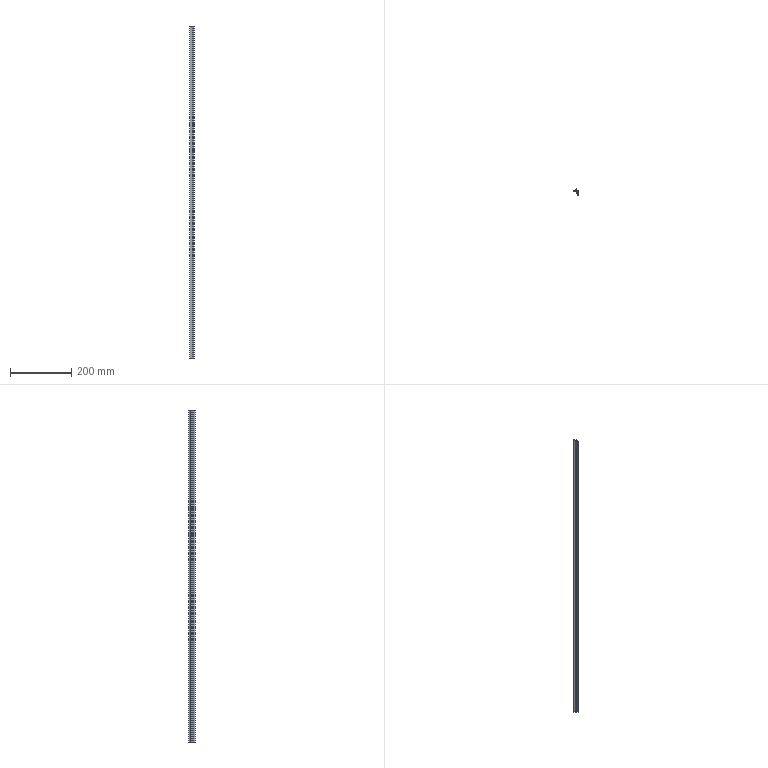Part | SolidWorks | features BaseBody 1, ICE 1, MoveFace 1 | 1 solid | 27 faces | box 14 x 20.3 x 1088 mm | volume 55396 mm3 | plane 20 | cylinder 7 | commonest cylinder face diameters 0.387 x2 0.8 x2 0.4 x1 20 x1 22 x1
STEP:
#1=CARTESIAN_POINT('',(-5.304,-0.625,200.));
#2=VERTEX_POINT('',#1);
#3=CARTESIAN_POINT('',(-5.449,-0.8125,200.));
#4=VERTEX_POINT('',#3);
#5=CARTESIAN_POINT('',(-5.255,-0.8125,200.));
#6=DIRECTION('',(0.,0.,1.));
#7=DIRECTION('',(-1.,0.,0.));
#8=AXIS2_PLACEMENT_3D('',#5,#6,#7);
#9=CIRCLE('',#8,0.1937);
#10=EDGE_CURVE('',#2,#4,#9,.T.);
#11=ORIENTED_EDGE('',*,*,#10,.T.);
#12=CARTESIAN_POINT('',(-5.449,-0.8125,-888.));
#13=VERTEX_POINT('',#12);
#14=CARTESIAN_POINT('',(-5.449,-0.8125,230.));
#15=DIRECTION('',(0.,0.,-1.));
#16=VECTOR('',#15,1000.);
#17=LINE('',#14,#16);
#18=EDGE_CURVE('',#4,#13,#17,.T.);
#19=ORIENTED_EDGE('',*,*,#18,.T.);
#20=CARTESIAN_POINT('',(-5.304,-0.625,-888.));
#21=VERTEX_POINT('',#20);
#22=CARTESIAN_POINT('',(-5.255,-0.8125,-888.));
#23=DIRECTION('',(0.,0.,-1.));
#24=DIRECTION('',(1.,0.,0.));
#25=AXIS2_PLACEMENT_3D('',#22,#23,#24);
#26=CIRCLE('',#25,0.1937);
#27=EDGE_CURVE('',#13,#21,#26,.T.);
#28=ORIENTED_EDGE('',*,*,#27,.T.);
#29=CARTESIAN_POINT('',(-5.304,-0.625,230.));
#30=DIRECTION('',(0.,0.,-1.));
#31=VECTOR('',#30,1000.);
#32=LINE('',#29,#31);
#33=EDGE_CURVE('',#2,#21,#32,.T.);
#34=ORIENTED_EDGE('',*,*,#33,.F.);
#35=EDGE_LOOP('',(#11,#19,#28,#34));
#36=FACE_OUTER_BOUND('',#35,.T.);
#37=CARTESIAN_POINT('',(-5.255,-0.8125,230.));
#38=DIRECTION('',(0.,0.,-1.));
#39=DIRECTION('',(-1.,0.,0.));
#40=AXIS2_PLACEMENT_3D('',#37,#38,#39);
#41=CYLINDRICAL_SURFACE('',#40,0.1937);
#42=ADVANCED_FACE('',(#36),#41,.F.);
#43=CARTESIAN_POINT('',(5.,-1.,-888.));
#44=VERTEX_POINT('',#43);
#45=CARTESIAN_POINT('',(5.,-14.3,-888.));
#46=VERTEX_POINT('',#45);
#47=CARTESIAN_POINT('',(5.,29.623,-888.));
#48=DIRECTION('',(0.,-1.,0.));
#49=VECTOR('',#48,1000.);
#50=LINE('',#47,#49);
#51=EDGE_CURVE('',#44,#46,#50,.T.);
#52=ORIENTED_EDGE('',*,*,#51,.F.);
#53=CARTESIAN_POINT('',(5.,-1.,200.));
#54=VERTEX_POINT('',#53);
#55=CARTESIAN_POINT('',(5.,-1.,230.));
#56=DIRECTION('',(0.,0.,-1.));
#57=VECTOR('',#56,1000.);
#58=LINE('',#55,#57);
#59=EDGE_CURVE('',#54,#44,#58,.T.);
#60=ORIENTED_EDGE('',*,*,#59,.F.);
#61=CARTESIAN_POINT('',(5.,-14.3,200.));
#62=VERTEX_POINT('',#61);
#63=CARTESIAN_POINT('',(5.,-14.3,200.));
#64=DIRECTION('',(0.,1.,0.));
#65=VECTOR('',#64,1000.);
#66=LINE('',#63,#65);
#67=EDGE_CURVE('',#62,#54,#66,.T.);
#68=ORIENTED_EDGE('',*,*,#67,.F.);
#69=CARTESIAN_POINT('',(5.,-14.3,230.));
#70=DIRECTION('',(0.,0.,1.));
#71=VECTOR('',#70,1000.);
#72=LINE('',#69,#71);
#73=EDGE_CURVE('',#46,#62,#72,.T.);
#74=ORIENTED_EDGE('',*,*,#73,.F.);
#75=EDGE_LOOP('',(#52,#60,#68,#74));
#76=FACE_OUTER_BOUND('',#75,.T.);
#77=CARTESIAN_POINT('',(5.,-14.3,230.));
#78=DIRECTION('',(-1.,0.,0.));
#79=DIRECTION('',(0.,0.,1.));
#80=AXIS2_PLACEMENT_3D('',#77,#78,#79);
#81=PLANE('',#80);
#82=ADVANCED_FACE('',(#76),#81,.F.);
#83=CARTESIAN_POINT('',(-9.,-2.,-888.));
#84=VERTEX_POINT('',#83);
#85=CARTESIAN_POINT('',(-9.,-2.,200.));
#86=VERTEX_POINT('',#85);
#87=CARTESIAN_POINT('',(-9.,-2.,230.));
#88=DIRECTION('',(0.,0.,1.));
#89=VECTOR('',#88,1000.);
#90=LINE('',#87,#89);
#91=EDGE_CURVE('',#84,#86,#90,.T.);
#92=ORIENTED_EDGE('',*,*,#91,.F.);
#93=CARTESIAN_POINT('',(0.9,-2.,-888.));
#94=VERTEX_POINT('',#93);
#95=CARTESIAN_POINT('',(5.,-2.,-888.));
#96=DIRECTION('',(-1.,0.,0.));
#97=VECTOR('',#96,1000.);
#98=LINE('',#95,#97);
#99=EDGE_CURVE('',#94,#84,#98,.T.);
#100=ORIENTED_EDGE('',*,*,#99,.F.);
#101=CARTESIAN_POINT('',(0.9,-2.,200.));
#102=VERTEX_POINT('',#101);
#103=CARTESIAN_POINT('',(0.9,-2.,230.));
#104=DIRECTION('',(0.,0.,-1.));
#105=VECTOR('',#104,1000.);
#106=LINE('',#103,#105);
#107=EDGE_CURVE('',#102,#94,#106,.T.);
#108=ORIENTED_EDGE('',*,*,#107,.F.);
#109=CARTESIAN_POINT('',(5.,-2.,200.));
#110=DIRECTION('',(1.,0.,0.));
#111=VECTOR('',#110,1000.);
#112=LINE('',#109,#111);
#113=EDGE_CURVE('',#86,#102,#112,.T.);
#114=ORIENTED_EDGE('',*,*,#113,.F.);
#115=EDGE_LOOP('',(#92,#100,#108,#114));
#116=FACE_OUTER_BOUND('',#115,.T.);
#117=CARTESIAN_POINT('',(-9.,-2.,230.));
#118=DIRECTION('',(0.,1.,0.));
#119=DIRECTION('',(0.,0.,1.));
#120=AXIS2_PLACEMENT_3D('',#117,#118,#119);
#121=PLANE('',#120);
#122=ADVANCED_FACE('',(#116),#121,.F.);
#123=CARTESIAN_POINT('',(4.,-6.,200.));
#124=VERTEX_POINT('',#123);
#125=CARTESIAN_POINT('',(4.,-3.,200.));
#126=VERTEX_POINT('',#125);
#127=CARTESIAN_POINT('',(4.,29.623,200.));
#128=DIRECTION('',(0.,1.,0.));
#129=VECTOR('',#128,1000.);
#130=LINE('',#127,#129);
#131=EDGE_CURVE('',#124,#126,#130,.T.);
#132=ORIENTED_EDGE('',*,*,#131,.F.);
#133=CARTESIAN_POINT('',(1.,-6.,200.));
#134=VERTEX_POINT('',#133);
#135=CARTESIAN_POINT('',(5.,-6.,200.));
#136=DIRECTION('',(1.,0.,0.));
#137=VECTOR('',#136,1000.);
#138=LINE('',#135,#137);
#139=EDGE_CURVE('',#134,#124,#138,.T.);
#140=ORIENTED_EDGE('',*,*,#139,.F.);
#141=CARTESIAN_POINT('',(1.,-6.7,200.));
#142=VERTEX_POINT('',#141);
#143=CARTESIAN_POINT('',(1.,-6.,200.));
#144=DIRECTION('',(0.,-1.,0.));
#145=VECTOR('',#144,1000.);
#146=LINE('',#143,#145);
#147=EDGE_CURVE('',#134,#142,#146,.T.);
#148=ORIENTED_EDGE('',*,*,#147,.T.);
#149=CARTESIAN_POINT('',(-1.7,-6.7,200.));
#150=VERTEX_POINT('',#149);
#151=CARTESIAN_POINT('',(5.,-6.7,200.));
#152=DIRECTION('',(1.,0.,0.));
#153=VECTOR('',#152,1000.);
#154=LINE('',#151,#153);
#155=EDGE_CURVE('',#150,#142,#154,.T.);
#156=ORIENTED_EDGE('',*,*,#155,.F.);
#157=CARTESIAN_POINT('',(-1.7,-7.7,200.));
#158=VERTEX_POINT('',#157);
#159=CARTESIAN_POINT('',(-1.7,-6.7,200.));
#160=DIRECTION('',(0.,-1.,0.));
#161=VECTOR('',#160,1000.);
#162=LINE('',#159,#161);
#163=EDGE_CURVE('',#150,#158,#162,.T.);
#164=ORIENTED_EDGE('',*,*,#163,.T.);
#165=CARTESIAN_POINT('',(4.,-7.7,200.));
#166=VERTEX_POINT('',#165);
#167=CARTESIAN_POINT('',(5.,-7.7,200.));
#168=DIRECTION('',(-1.,0.,0.));
#169=VECTOR('',#168,1000.);
#170=LINE('',#167,#169);
#171=EDGE_CURVE('',#166,#158,#170,.T.);
#172=ORIENTED_EDGE('',*,*,#171,.F.);
#173=CARTESIAN_POINT('',(4.,-14.3,200.));
#174=VERTEX_POINT('',#173);
#175=CARTESIAN_POINT('',(4.,29.623,200.));
#176=DIRECTION('',(0.,1.,0.));
#177=VECTOR('',#176,1000.);
#178=LINE('',#175,#177);
#179=EDGE_CURVE('',#174,#166,#178,.T.);
#180=ORIENTED_EDGE('',*,*,#179,.F.);
#181=CARTESIAN_POINT('',(5.,-14.3,200.));
#182=DIRECTION('',(-1.,0.,0.));
#183=VECTOR('',#182,1000.);
#184=LINE('',#181,#183);
#185=EDGE_CURVE('',#62,#174,#184,.T.);
#186=ORIENTED_EDGE('',*,*,#185,.F.);
#187=ORIENTED_EDGE('',*,*,#67,.T.);
#188=CARTESIAN_POINT('',(-5.207,-1.,200.));
#189=VERTEX_POINT('',#188);
#190=CARTESIAN_POINT('',(5.,-1.,200.));
#191=DIRECTION('',(1.,0.,0.));
#192=VECTOR('',#191,1000.);
#193=LINE('',#190,#192);
#194=EDGE_CURVE('',#189,#54,#193,.T.);
#195=ORIENTED_EDGE('',*,*,#194,.F.);
#196=CARTESIAN_POINT('',(-5.255,-0.8125,200.));
#197=DIRECTION('',(0.,0.,1.));
#198=DIRECTION('',(-1.,0.,0.));
#199=AXIS2_PLACEMENT_3D('',#196,#197,#198);
#200=CIRCLE('',#199,0.1937);
#201=EDGE_CURVE('',#4,#189,#200,.T.);
#202=ORIENTED_EDGE('',*,*,#201,.F.);
#203=ORIENTED_EDGE('',*,*,#10,.F.);
#204=CARTESIAN_POINT('',(-1.368,3.063,200.));
#205=VERTEX_POINT('',#204);
#206=CARTESIAN_POINT('',(-10.628,9.,200.));
#207=DIRECTION('',(0.,0.,1.));
#208=DIRECTION('',(-1.,0.,0.));
#209=AXIS2_PLACEMENT_3D('',#206,#207,#208);
#210=CIRCLE('',#209,11.);
#211=EDGE_CURVE('',#2,#205,#210,.T.);
#212=ORIENTED_EDGE('',*,*,#211,.T.);
#213=CARTESIAN_POINT('',(-1.,2.955,200.));
#214=VERTEX_POINT('',#213);
#215=CARTESIAN_POINT('',(-1.2,2.955,200.));
#216=DIRECTION('',(0.,0.,1.));
#217=DIRECTION('',(-1.,0.,0.));
#218=AXIS2_PLACEMENT_3D('',#215,#216,#217);
#219=CIRCLE('',#218,0.2);
#220=EDGE_CURVE('',#214,#205,#219,.T.);
#221=ORIENTED_EDGE('',*,*,#220,.F.);
#222=CARTESIAN_POINT('',(-1.,1.5,200.));
#223=VERTEX_POINT('',#222);
#224=CARTESIAN_POINT('',(-1.,2.955,200.));
#225=DIRECTION('',(0.,1.,0.));
#226=VECTOR('',#225,1000.);
#227=LINE('',#224,#226);
#228=EDGE_CURVE('',#223,#214,#227,.T.);
#229=ORIENTED_EDGE('',*,*,#228,.F.);
#230=CARTESIAN_POINT('',(0.,1.5,200.));
#231=VERTEX_POINT('',#230);
#232=CARTESIAN_POINT('',(-1.,1.5,200.));
#233=DIRECTION('',(-1.,0.,0.));
#234=VECTOR('',#233,1000.);
#235=LINE('',#232,#234);
#236=EDGE_CURVE('',#231,#223,#235,.T.);
#237=ORIENTED_EDGE('',*,*,#236,.F.);
#238=CARTESIAN_POINT('',(0.,6.,200.));
#239=VERTEX_POINT('',#238);
#240=CARTESIAN_POINT('',(0.,1.5,200.));
#241=DIRECTION('',(0.,-1.,0.));
#242=VECTOR('',#241,1000.);
#243=LINE('',#240,#242);
#244=EDGE_CURVE('',#239,#231,#243,.T.);
#245=ORIENTED_EDGE('',*,*,#244,.F.);
#246=CARTESIAN_POINT('',(-0.8,6.,200.));
#247=VERTEX_POINT('',#246);
#248=CARTESIAN_POINT('',(0.,6.,200.));
#249=DIRECTION('',(1.,0.,0.));
#250=VECTOR('',#249,1000.);
#251=LINE('',#248,#250);
#252=EDGE_CURVE('',#247,#239,#251,.T.);
#253=ORIENTED_EDGE('',*,*,#252,.F.);
#254=CARTESIAN_POINT('',(-1.178,5.731,200.));
#255=VERTEX_POINT('',#254);
#256=CARTESIAN_POINT('',(-0.8,5.6,200.));
#257=DIRECTION('',(0.,0.,1.));
#258=DIRECTION('',(-1.,0.,0.));
#259=AXIS2_PLACEMENT_3D('',#256,#257,#258);
#260=CIRCLE('',#259,0.4);
#261=EDGE_CURVE('',#247,#255,#260,.T.);
#262=ORIENTED_EDGE('',*,*,#261,.T.);
#263=CARTESIAN_POINT('',(-8.678,-0.8077,200.));
#264=VERTEX_POINT('',#263);
#265=CARTESIAN_POINT('',(-10.628,9.,200.));
#266=DIRECTION('',(0.,0.,1.));
#267=DIRECTION('',(-1.,0.,0.));
#268=AXIS2_PLACEMENT_3D('',#265,#266,#267);
#269=CIRCLE('',#268,10.);
#270=EDGE_CURVE('',#264,#255,#269,.T.);
#271=ORIENTED_EDGE('',*,*,#270,.F.);
#272=CARTESIAN_POINT('',(-9.,-1.2,200.));
#273=VERTEX_POINT('',#272);
#274=CARTESIAN_POINT('',(-8.6,-1.2,200.));
#275=DIRECTION('',(0.,0.,1.));
#276=DIRECTION('',(-1.,0.,0.));
#277=AXIS2_PLACEMENT_3D('',#274,#275,#276);
#278=CIRCLE('',#277,0.4);
#279=EDGE_CURVE('',#264,#273,#278,.T.);
#280=ORIENTED_EDGE('',*,*,#279,.T.);
#281=CARTESIAN_POINT('',(-9.,8.,200.));
#282=DIRECTION('',(0.,-1.,0.));
#283=VECTOR('',#282,1000.);
#284=LINE('',#281,#283);
#285=EDGE_CURVE('',#273,#86,#284,.T.);
#286=ORIENTED_EDGE('',*,*,#285,.T.);
#287=ORIENTED_EDGE('',*,*,#113,.T.);
#288=CARTESIAN_POINT('',(0.9,-3.,200.));
#289=VERTEX_POINT('',#288);
#290=CARTESIAN_POINT('',(0.9,29.623,200.));
#291=DIRECTION('',(0.,1.,0.));
#292=VECTOR('',#291,1000.);
#293=LINE('',#290,#292);
#294=EDGE_CURVE('',#289,#102,#293,.T.);
#295=ORIENTED_EDGE('',*,*,#294,.F.);
#296=CARTESIAN_POINT('',(5.,-3.,200.));
#297=DIRECTION('',(-1.,0.,0.));
#298=VECTOR('',#297,1000.);
#299=LINE('',#296,#298);
#300=EDGE_CURVE('',#126,#289,#299,.T.);
#301=ORIENTED_EDGE('',*,*,#300,.F.);
#302=EDGE_LOOP('',(#132,#140,#148,#156,#164,#172,#180,#186,#187,#195,#202,#203,#212,#221,#229,#237,#245,#253,#262,#271,#280,#286,#287,#295,#301));
#303=FACE_OUTER_BOUND('',#302,.T.);
#304=CARTESIAN_POINT('',(5.,29.623,200.));
#305=DIRECTION('',(0.,0.,-1.));
#306=DIRECTION('',(-1.,0.,0.));
#307=AXIS2_PLACEMENT_3D('',#304,#305,#306);
#308=PLANE('',#307);
#309=ADVANCED_FACE('',(#303),#308,.F.);
#310=ORIENTED_EDGE('',*,*,#185,.T.);
#311=CARTESIAN_POINT('',(4.,-14.3,-888.));
#312=VERTEX_POINT('',#311);
#313=CARTESIAN_POINT('',(4.,-14.3,230.));
#314=DIRECTION('',(0.,0.,1.));
#315=VECTOR('',#314,1000.);
#316=LINE('',#313,#315);
#317=EDGE_CURVE('',#312,#174,#316,.T.);
#318=ORIENTED_EDGE('',*,*,#317,.F.);
#319=CARTESIAN_POINT('',(5.,-14.3,-888.));
#320=DIRECTION('',(-1.,0.,0.));
#321=VECTOR('',#320,1000.);
#322=LINE('',#319,#321);
#323=EDGE_CURVE('',#46,#312,#322,.T.);
#324=ORIENTED_EDGE('',*,*,#323,.F.);
#325=ORIENTED_EDGE('',*,*,#73,.T.);
#326=EDGE_LOOP('',(#310,#318,#324,#325));
#327=FACE_OUTER_BOUND('',#326,.T.);
#328=CARTESIAN_POINT('',(4.,-14.3,230.));
#329=DIRECTION('',(0.,1.,0.));
#330=DIRECTION('',(0.,0.,1.));
#331=AXIS2_PLACEMENT_3D('',#328,#329,#330);
#332=PLANE('',#331);
#333=ADVANCED_FACE('',(#327),#332,.F.);
#334=ORIENTED_EDGE('',*,*,#51,.T.);
#335=ORIENTED_EDGE('',*,*,#323,.T.);
#336=CARTESIAN_POINT('',(4.,-7.7,-888.));
#337=VERTEX_POINT('',#336);
#338=CARTESIAN_POINT('',(4.,-7.7,-888.));
#339=DIRECTION('',(0.,-1.,0.));
#340=VECTOR('',#339,1000.);
#341=LINE('',#338,#340);
#342=EDGE_CURVE('',#337,#312,#341,.T.);
#343=ORIENTED_EDGE('',*,*,#342,.F.);
#344=CARTESIAN_POINT('',(-1.7,-7.7,-888.));
#345=VERTEX_POINT('',#344);
#346=CARTESIAN_POINT('',(-1.7,-7.7,-888.));
#347=DIRECTION('',(1.,0.,0.));
#348=VECTOR('',#347,1000.);
#349=LINE('',#346,#348);
#350=EDGE_CURVE('',#345,#337,#349,.T.);
#351=ORIENTED_EDGE('',*,*,#350,.F.);
#352=CARTESIAN_POINT('',(-1.7,-6.7,-888.));
#353=VERTEX_POINT('',#352);
#354=CARTESIAN_POINT('',(-1.7,29.623,-888.));
#355=DIRECTION('',(0.,1.,0.));
#356=VECTOR('',#355,1000.);
#357=LINE('',#354,#356);
#358=EDGE_CURVE('',#345,#353,#357,.T.);
#359=ORIENTED_EDGE('',*,*,#358,.T.);
#360=CARTESIAN_POINT('',(1.,-6.7,-888.));
#361=VERTEX_POINT('',#360);
#362=CARTESIAN_POINT('',(1.,-6.7,-888.));
#363=DIRECTION('',(-1.,0.,0.));
#364=VECTOR('',#363,1000.);
#365=LINE('',#362,#364);
#366=EDGE_CURVE('',#361,#353,#365,.T.);
#367=ORIENTED_EDGE('',*,*,#366,.F.);
#368=CARTESIAN_POINT('',(1.,-6.,-888.));
#369=VERTEX_POINT('',#368);
#370=CARTESIAN_POINT('',(1.,29.623,-888.));
#371=DIRECTION('',(0.,1.,0.));
#372=VECTOR('',#371,1000.);
#373=LINE('',#370,#372);
#374=EDGE_CURVE('',#361,#369,#373,.T.);
#375=ORIENTED_EDGE('',*,*,#374,.T.);
#376=CARTESIAN_POINT('',(4.,-6.,-888.));
#377=VERTEX_POINT('',#376);
#378=CARTESIAN_POINT('',(4.,-6.,-888.));
#379=DIRECTION('',(-1.,0.,0.));
#380=VECTOR('',#379,1000.);
#381=LINE('',#378,#380);
#382=EDGE_CURVE('',#377,#369,#381,.T.);
#383=ORIENTED_EDGE('',*,*,#382,.F.);
#384=CARTESIAN_POINT('',(4.,-3.,-888.));
#385=VERTEX_POINT('',#384);
#386=CARTESIAN_POINT('',(4.,-3.,-888.));
#387=DIRECTION('',(0.,-1.,0.));
#388=VECTOR('',#387,1000.);
#389=LINE('',#386,#388);
#390=EDGE_CURVE('',#385,#377,#389,.T.);
#391=ORIENTED_EDGE('',*,*,#390,.F.);
#392=CARTESIAN_POINT('',(0.9,-3.,-888.));
#393=VERTEX_POINT('',#392);
#394=CARTESIAN_POINT('',(0.9,-3.,-888.));
#395=DIRECTION('',(1.,0.,0.));
#396=VECTOR('',#395,1000.);
#397=LINE('',#394,#396);
#398=EDGE_CURVE('',#393,#385,#397,.T.);
#399=ORIENTED_EDGE('',*,*,#398,.F.);
#400=CARTESIAN_POINT('',(0.9,-2.,-888.));
#401=DIRECTION('',(0.,-1.,0.));
#402=VECTOR('',#401,1000.);
#403=LINE('',#400,#402);
#404=EDGE_CURVE('',#94,#393,#403,.T.);
#405=ORIENTED_EDGE('',*,*,#404,.F.);
#406=ORIENTED_EDGE('',*,*,#99,.T.);
#407=CARTESIAN_POINT('',(-9.,-1.2,-888.));
#408=VERTEX_POINT('',#407);
#409=CARTESIAN_POINT('',(-9.,-1.2,-888.));
#410=DIRECTION('',(0.,-1.,0.));
#411=VECTOR('',#410,1000.);
#412=LINE('',#409,#411);
#413=EDGE_CURVE('',#408,#84,#412,.T.);
#414=ORIENTED_EDGE('',*,*,#413,.F.);
#415=CARTESIAN_POINT('',(-8.678,-0.8077,-888.));
#416=VERTEX_POINT('',#415);
#417=CARTESIAN_POINT('',(-8.6,-1.2,-888.));
#418=DIRECTION('',(0.,0.,-1.));
#419=DIRECTION('',(1.,0.,0.));
#420=AXIS2_PLACEMENT_3D('',#417,#418,#419);
#421=CIRCLE('',#420,0.4);
#422=EDGE_CURVE('',#408,#416,#421,.T.);
#423=ORIENTED_EDGE('',*,*,#422,.T.);
#424=CARTESIAN_POINT('',(-1.178,5.731,-888.));
#425=VERTEX_POINT('',#424);
#426=CARTESIAN_POINT('',(-10.628,9.,-888.));
#427=DIRECTION('',(0.,0.,-1.));
#428=DIRECTION('',(1.,0.,0.));
#429=AXIS2_PLACEMENT_3D('',#426,#427,#428);
#430=CIRCLE('',#429,10.);
#431=EDGE_CURVE('',#425,#416,#430,.T.);
#432=ORIENTED_EDGE('',*,*,#431,.F.);
#433=CARTESIAN_POINT('',(-0.8,6.,-888.));
#434=VERTEX_POINT('',#433);
#435=CARTESIAN_POINT('',(-0.8,5.6,-888.));
#436=DIRECTION('',(0.,0.,-1.));
#437=DIRECTION('',(1.,0.,0.));
#438=AXIS2_PLACEMENT_3D('',#435,#436,#437);
#439=CIRCLE('',#438,0.4);
#440=EDGE_CURVE('',#425,#434,#439,.T.);
#441=ORIENTED_EDGE('',*,*,#440,.T.);
#442=CARTESIAN_POINT('',(0.,6.,-888.));
#443=VERTEX_POINT('',#442);
#444=CARTESIAN_POINT('',(0.,6.,-888.));
#445=DIRECTION('',(-1.,0.,0.));
#446=VECTOR('',#445,1000.);
#447=LINE('',#444,#446);
#448=EDGE_CURVE('',#443,#434,#447,.T.);
#449=ORIENTED_EDGE('',*,*,#448,.F.);
#450=CARTESIAN_POINT('',(0.,1.5,-888.));
#451=VERTEX_POINT('',#450);
#452=CARTESIAN_POINT('',(0.,1.5,-888.));
#453=DIRECTION('',(0.,1.,0.));
#454=VECTOR('',#453,1000.);
#455=LINE('',#452,#454);
#456=EDGE_CURVE('',#451,#443,#455,.T.);
#457=ORIENTED_EDGE('',*,*,#456,.F.);
#458=CARTESIAN_POINT('',(-1.,1.5,-888.));
#459=VERTEX_POINT('',#458);
#460=CARTESIAN_POINT('',(-1.,1.5,-888.));
#461=DIRECTION('',(1.,0.,0.));
#462=VECTOR('',#461,1000.);
#463=LINE('',#460,#462);
#464=EDGE_CURVE('',#459,#451,#463,.T.);
#465=ORIENTED_EDGE('',*,*,#464,.F.);
#466=CARTESIAN_POINT('',(-1.,2.955,-888.));
#467=VERTEX_POINT('',#466);
#468=CARTESIAN_POINT('',(-1.,2.955,-888.));
#469=DIRECTION('',(0.,-1.,0.));
#470=VECTOR('',#469,1000.);
#471=LINE('',#468,#470);
#472=EDGE_CURVE('',#467,#459,#471,.T.);
#473=ORIENTED_EDGE('',*,*,#472,.F.);
#474=CARTESIAN_POINT('',(-1.368,3.063,-888.));
#475=VERTEX_POINT('',#474);
#476=CARTESIAN_POINT('',(-1.2,2.955,-888.));
#477=DIRECTION('',(0.,0.,-1.));
#478=DIRECTION('',(1.,0.,0.));
#479=AXIS2_PLACEMENT_3D('',#476,#477,#478);
#480=CIRCLE('',#479,0.2);
#481=EDGE_CURVE('',#475,#467,#480,.T.);
#482=ORIENTED_EDGE('',*,*,#481,.F.);
#483=CARTESIAN_POINT('',(-10.628,9.,-888.));
#484=DIRECTION('',(0.,0.,-1.));
#485=DIRECTION('',(1.,0.,0.));
#486=AXIS2_PLACEMENT_3D('',#483,#484,#485);
#487=CIRCLE('',#486,11.);
#488=EDGE_CURVE('',#475,#21,#487,.T.);
#489=ORIENTED_EDGE('',*,*,#488,.T.);
#490=ORIENTED_EDGE('',*,*,#27,.F.);
#491=CARTESIAN_POINT('',(-5.207,-1.,-888.));
#492=VERTEX_POINT('',#491);
#493=CARTESIAN_POINT('',(-5.255,-0.8125,-888.));
#494=DIRECTION('',(0.,0.,-1.));
#495=DIRECTION('',(1.,0.,0.));
#496=AXIS2_PLACEMENT_3D('',#493,#494,#495);
#497=CIRCLE('',#496,0.1937);
#498=EDGE_CURVE('',#492,#13,#497,.T.);
#499=ORIENTED_EDGE('',*,*,#498,.F.);
#500=CARTESIAN_POINT('',(5.,-1.,-888.));
#501=DIRECTION('',(-1.,0.,0.));
#502=VECTOR('',#501,1000.);
#503=LINE('',#500,#502);
#504=EDGE_CURVE('',#44,#492,#503,.T.);
#505=ORIENTED_EDGE('',*,*,#504,.F.);
#506=EDGE_LOOP('',(#334,#335,#343,#351,#359,#367,#375,#383,#391,#399,#405,#406,#414,#423,#432,#441,#449,#457,#465,#473,#482,#489,#490,#499,#505));
#507=FACE_OUTER_BOUND('',#506,.T.);
#508=CARTESIAN_POINT('',(5.,29.623,-888.));
#509=DIRECTION('',(0.,0.,1.));
#510=DIRECTION('',(1.,0.,0.));
#511=AXIS2_PLACEMENT_3D('',#508,#509,#510);
#512=PLANE('',#511);
#513=ADVANCED_FACE('',(#507),#512,.F.);
#514=ORIENTED_EDGE('',*,*,#59,.T.);
#515=ORIENTED_EDGE('',*,*,#504,.T.);
#516=CARTESIAN_POINT('',(-5.207,-1.,230.));
#517=DIRECTION('',(0.,0.,-1.));
#518=VECTOR('',#517,1000.);
#519=LINE('',#516,#518);
#520=EDGE_CURVE('',#189,#492,#519,.T.);
#521=ORIENTED_EDGE('',*,*,#520,.F.);
#522=ORIENTED_EDGE('',*,*,#194,.T.);
#523=EDGE_LOOP('',(#514,#515,#521,#522));
#524=FACE_OUTER_BOUND('',#523,.T.);
#525=CARTESIAN_POINT('',(5.,-1.,230.));
#526=DIRECTION('',(0.,-1.,0.));
#527=DIRECTION('',(0.,0.,-1.));
#528=AXIS2_PLACEMENT_3D('',#525,#526,#527);
#529=PLANE('',#528);
#530=ADVANCED_FACE('',(#524),#529,.F.);
#531=CARTESIAN_POINT('',(-9.,-1.2,230.));
#532=DIRECTION('',(0.,0.,1.));
#533=VECTOR('',#532,1000.);
#534=LINE('',#531,#533);
#535=EDGE_CURVE('',#408,#273,#534,.T.);
#536=ORIENTED_EDGE('',*,*,#535,.F.);
#537=ORIENTED_EDGE('',*,*,#413,.T.);
#538=ORIENTED_EDGE('',*,*,#91,.T.);
#539=ORIENTED_EDGE('',*,*,#285,.F.);
#540=EDGE_LOOP('',(#536,#537,#538,#539));
#541=FACE_OUTER_BOUND('',#540,.T.);
#542=CARTESIAN_POINT('',(-9.,-1.2,230.));
#543=DIRECTION('',(1.,0.,0.));
#544=DIRECTION('',(0.,0.,-1.));
#545=AXIS2_PLACEMENT_3D('',#542,#543,#544);
#546=PLANE('',#545);
#547=ADVANCED_FACE('',(#541),#546,.F.);
#548=ORIENTED_EDGE('',*,*,#294,.T.);
#549=ORIENTED_EDGE('',*,*,#107,.T.);
#550=ORIENTED_EDGE('',*,*,#404,.T.);
#551=CARTESIAN_POINT('',(0.9,-3.,230.));
#552=DIRECTION('',(0.,0.,-1.));
#553=VECTOR('',#552,1000.);
#554=LINE('',#551,#553);
#555=EDGE_CURVE('',#289,#393,#554,.T.);
#556=ORIENTED_EDGE('',*,*,#555,.F.);
#557=EDGE_LOOP('',(#548,#549,#550,#556));
#558=FACE_OUTER_BOUND('',#557,.T.);
#559=CARTESIAN_POINT('',(0.9,-2.,230.));
#560=DIRECTION('',(1.,0.,0.));
#561=DIRECTION('',(0.,0.,-1.));
#562=AXIS2_PLACEMENT_3D('',#559,#560,#561);
#563=PLANE('',#562);
#564=ADVANCED_FACE('',(#558),#563,.F.);
#565=ORIENTED_EDGE('',*,*,#300,.T.);
#566=ORIENTED_EDGE('',*,*,#555,.T.);
#567=ORIENTED_EDGE('',*,*,#398,.T.);
#568=CARTESIAN_POINT('',(4.,-3.,230.));
#569=DIRECTION('',(0.,0.,-1.));
#570=VECTOR('',#569,1000.);
#571=LINE('',#568,#570);
#572=EDGE_CURVE('',#126,#385,#571,.T.);
#573=ORIENTED_EDGE('',*,*,#572,.F.);
#574=EDGE_LOOP('',(#565,#566,#567,#573));
#575=FACE_OUTER_BOUND('',#574,.T.);
#576=CARTESIAN_POINT('',(0.9,-3.,230.));
#577=DIRECTION('',(0.,1.,0.));
#578=DIRECTION('',(0.,0.,1.));
#579=AXIS2_PLACEMENT_3D('',#576,#577,#578);
#580=PLANE('',#579);
#581=ADVANCED_FACE('',(#575),#580,.F.);
#582=ORIENTED_EDGE('',*,*,#131,.T.);
#583=ORIENTED_EDGE('',*,*,#572,.T.);
#584=ORIENTED_EDGE('',*,*,#390,.T.);
#585=CARTESIAN_POINT('',(4.,-6.,230.));
#586=DIRECTION('',(0.,0.,-1.));
#587=VECTOR('',#586,1000.);
#588=LINE('',#585,#587);
#589=EDGE_CURVE('',#124,#377,#588,.T.);
#590=ORIENTED_EDGE('',*,*,#589,.F.);
#591=EDGE_LOOP('',(#582,#583,#584,#590));
#592=FACE_OUTER_BOUND('',#591,.T.);
#593=CARTESIAN_POINT('',(4.,-3.,230.));
#594=DIRECTION('',(1.,0.,0.));
#595=DIRECTION('',(0.,0.,-1.));
#596=AXIS2_PLACEMENT_3D('',#593,#594,#595);
#597=PLANE('',#596);
#598=ADVANCED_FACE('',(#592),#597,.F.);
#599=ORIENTED_EDGE('',*,*,#139,.T.);
#600=ORIENTED_EDGE('',*,*,#589,.T.);
#601=ORIENTED_EDGE('',*,*,#382,.T.);
#602=CARTESIAN_POINT('',(1.,-6.,230.));
#603=DIRECTION('',(0.,0.,-1.));
#604=VECTOR('',#603,1000.);
#605=LINE('',#602,#604);
#606=EDGE_CURVE('',#134,#369,#605,.T.);
#607=ORIENTED_EDGE('',*,*,#606,.F.);
#608=EDGE_LOOP('',(#599,#600,#601,#607));
#609=FACE_OUTER_BOUND('',#608,.T.);
#610=CARTESIAN_POINT('',(4.,-6.,230.));
#611=DIRECTION('',(0.,-1.,0.));
#612=DIRECTION('',(0.,0.,-1.));
#613=AXIS2_PLACEMENT_3D('',#610,#611,#612);
#614=PLANE('',#613);
#615=ADVANCED_FACE('',(#609),#614,.F.);
#616=ORIENTED_EDGE('',*,*,#155,.T.);
#617=CARTESIAN_POINT('',(1.,-6.7,230.));
#618=DIRECTION('',(0.,0.,1.));
#619=VECTOR('',#618,1000.);
#620=LINE('',#617,#619);
#621=EDGE_CURVE('',#361,#142,#620,.T.);
#622=ORIENTED_EDGE('',*,*,#621,.F.);
#623=ORIENTED_EDGE('',*,*,#366,.T.);
#624=CARTESIAN_POINT('',(-1.7,-6.7,230.));
#625=DIRECTION('',(0.,0.,-1.));
#626=VECTOR('',#625,1000.);
#627=LINE('',#624,#626);
#628=EDGE_CURVE('',#150,#353,#627,.T.);
#629=ORIENTED_EDGE('',*,*,#628,.F.);
#630=EDGE_LOOP('',(#616,#622,#623,#629));
#631=FACE_OUTER_BOUND('',#630,.T.);
#632=CARTESIAN_POINT('',(1.,-6.7,230.));
#633=DIRECTION('',(0.,-1.,0.));
#634=DIRECTION('',(0.,0.,-1.));
#635=AXIS2_PLACEMENT_3D('',#632,#633,#634);
#636=PLANE('',#635);
#637=ADVANCED_FACE('',(#631),#636,.F.);
#638=ORIENTED_EDGE('',*,*,#171,.T.);
#639=CARTESIAN_POINT('',(-1.7,-7.7,230.));
#640=DIRECTION('',(0.,0.,1.));
#641=VECTOR('',#640,1000.);
#642=LINE('',#639,#641);
#643=EDGE_CURVE('',#345,#158,#642,.T.);
#644=ORIENTED_EDGE('',*,*,#643,.F.);
#645=ORIENTED_EDGE('',*,*,#350,.T.);
#646=CARTESIAN_POINT('',(4.,-7.7,230.));
#647=DIRECTION('',(0.,0.,-1.));
#648=VECTOR('',#647,1000.);
#649=LINE('',#646,#648);
#650=EDGE_CURVE('',#166,#337,#649,.T.);
#651=ORIENTED_EDGE('',*,*,#650,.F.);
#652=EDGE_LOOP('',(#638,#644,#645,#651));
#653=FACE_OUTER_BOUND('',#652,.T.);
#654=CARTESIAN_POINT('',(-1.7,-7.7,230.));
#655=DIRECTION('',(0.,1.,0.));
#656=DIRECTION('',(0.,0.,1.));
#657=AXIS2_PLACEMENT_3D('',#654,#655,#656);
#658=PLANE('',#657);
#659=ADVANCED_FACE('',(#653),#658,.F.);
#660=ORIENTED_EDGE('',*,*,#179,.T.);
#661=ORIENTED_EDGE('',*,*,#650,.T.);
#662=ORIENTED_EDGE('',*,*,#342,.T.);
#663=ORIENTED_EDGE('',*,*,#317,.T.);
#664=EDGE_LOOP('',(#660,#661,#662,#663));
#665=FACE_OUTER_BOUND('',#664,.T.);
#666=CARTESIAN_POINT('',(4.,-7.7,230.));
#667=DIRECTION('',(1.,0.,0.));
#668=DIRECTION('',(0.,0.,-1.));
#669=AXIS2_PLACEMENT_3D('',#666,#667,#668);
#670=PLANE('',#669);
#671=ADVANCED_FACE('',(#665),#670,.F.);
#672=ORIENTED_EDGE('',*,*,#18,.F.);
#673=ORIENTED_EDGE('',*,*,#201,.T.);
#674=ORIENTED_EDGE('',*,*,#520,.T.);
#675=ORIENTED_EDGE('',*,*,#498,.T.);
#676=EDGE_LOOP('',(#672,#673,#674,#675));
#677=FACE_OUTER_BOUND('',#676,.T.);
#678=CARTESIAN_POINT('',(-5.255,-0.8125,230.));
#679=DIRECTION('',(0.,0.,-1.));
#680=DIRECTION('',(-1.,0.,0.));
#681=AXIS2_PLACEMENT_3D('',#678,#679,#680);
#682=CYLINDRICAL_SURFACE('',#681,0.1937);
#683=ADVANCED_FACE('',(#677),#682,.F.);
#684=CARTESIAN_POINT('',(-1.,2.955,230.));
#685=DIRECTION('',(0.,0.,1.));
#686=VECTOR('',#685,1000.);
#687=LINE('',#684,#686);
#688=EDGE_CURVE('',#467,#214,#687,.T.);
#689=ORIENTED_EDGE('',*,*,#688,.F.);
#690=ORIENTED_EDGE('',*,*,#472,.T.);
#691=CARTESIAN_POINT('',(-1.,1.5,230.));
#692=DIRECTION('',(0.,0.,-1.));
#693=VECTOR('',#692,1000.);
#694=LINE('',#691,#693);
#695=EDGE_CURVE('',#223,#459,#694,.T.);
#696=ORIENTED_EDGE('',*,*,#695,.F.);
#697=ORIENTED_EDGE('',*,*,#228,.T.);
#698=EDGE_LOOP('',(#689,#690,#696,#697));
#699=FACE_OUTER_BOUND('',#698,.T.);
#700=CARTESIAN_POINT('',(-1.,2.955,230.));
#701=DIRECTION('',(1.,0.,0.));
#702=DIRECTION('',(0.,0.,-1.));
#703=AXIS2_PLACEMENT_3D('',#700,#701,#702);
#704=PLANE('',#703);
#705=ADVANCED_FACE('',(#699),#704,.F.);
#706=ORIENTED_EDGE('',*,*,#488,.F.);
#707=CARTESIAN_POINT('',(-1.368,3.063,230.));
#708=DIRECTION('',(0.,0.,1.));
#709=VECTOR('',#708,1000.);
#710=LINE('',#707,#709);
#711=EDGE_CURVE('',#475,#205,#710,.T.);
#712=ORIENTED_EDGE('',*,*,#711,.T.);
#713=ORIENTED_EDGE('',*,*,#211,.F.);
#714=ORIENTED_EDGE('',*,*,#33,.T.);
#715=EDGE_LOOP('',(#706,#712,#713,#714));
#716=FACE_OUTER_BOUND('',#715,.T.);
#717=CARTESIAN_POINT('',(-10.628,9.,230.));
#718=DIRECTION('',(0.,0.,-1.));
#719=DIRECTION('',(-1.,0.,0.));
#720=AXIS2_PLACEMENT_3D('',#717,#718,#719);
#721=CYLINDRICAL_SURFACE('',#720,11.);
#722=ADVANCED_FACE('',(#716),#721,.T.);
#723=CARTESIAN_POINT('',(-1.178,5.731,230.));
#724=DIRECTION('',(0.,0.,1.));
#725=VECTOR('',#724,1000.);
#726=LINE('',#723,#725);
#727=EDGE_CURVE('',#425,#255,#726,.T.);
#728=ORIENTED_EDGE('',*,*,#727,.F.);
#729=ORIENTED_EDGE('',*,*,#431,.T.);
#730=CARTESIAN_POINT('',(-8.678,-0.8077,230.));
#731=DIRECTION('',(0.,0.,-1.));
#732=VECTOR('',#731,1000.);
#733=LINE('',#730,#732);
#734=EDGE_CURVE('',#264,#416,#733,.T.);
#735=ORIENTED_EDGE('',*,*,#734,.F.);
#736=ORIENTED_EDGE('',*,*,#270,.T.);
#737=EDGE_LOOP('',(#728,#729,#735,#736));
#738=FACE_OUTER_BOUND('',#737,.T.);
#739=CARTESIAN_POINT('',(-10.628,9.,230.));
#740=DIRECTION('',(0.,0.,-1.));
#741=DIRECTION('',(-1.,0.,0.));
#742=AXIS2_PLACEMENT_3D('',#739,#740,#741);
#743=CYLINDRICAL_SURFACE('',#742,10.);
#744=ADVANCED_FACE('',(#738),#743,.F.);
#745=CARTESIAN_POINT('',(0.,1.5,230.));
#746=DIRECTION('',(0.,0.,1.));
#747=VECTOR('',#746,1000.);
#748=LINE('',#745,#747);
#749=EDGE_CURVE('',#451,#231,#748,.T.);
#750=ORIENTED_EDGE('',*,*,#749,.F.);
#751=ORIENTED_EDGE('',*,*,#456,.T.);
#752=CARTESIAN_POINT('',(0.,6.,230.));
#753=DIRECTION('',(0.,0.,-1.));
#754=VECTOR('',#753,1000.);
#755=LINE('',#752,#754);
#756=EDGE_CURVE('',#239,#443,#755,.T.);
#757=ORIENTED_EDGE('',*,*,#756,.F.);
#758=ORIENTED_EDGE('',*,*,#244,.T.);
#759=EDGE_LOOP('',(#750,#751,#757,#758));
#760=FACE_OUTER_BOUND('',#759,.T.);
#761=CARTESIAN_POINT('',(0.,1.5,230.));
#762=DIRECTION('',(-1.,0.,0.));
#763=DIRECTION('',(0.,0.,1.));
#764=AXIS2_PLACEMENT_3D('',#761,#762,#763);
#765=PLANE('',#764);
#766=ADVANCED_FACE('',(#760),#765,.F.);
#767=ORIENTED_EDGE('',*,*,#422,.F.);
#768=ORIENTED_EDGE('',*,*,#535,.T.);
#769=ORIENTED_EDGE('',*,*,#279,.F.);
#770=ORIENTED_EDGE('',*,*,#734,.T.);
#771=EDGE_LOOP('',(#767,#768,#769,#770));
#772=FACE_OUTER_BOUND('',#771,.T.);
#773=CARTESIAN_POINT('',(-8.6,-1.2,230.));
#774=DIRECTION('',(0.,0.,-1.));
#775=DIRECTION('',(-1.,0.,0.));
#776=AXIS2_PLACEMENT_3D('',#773,#774,#775);
#777=CYLINDRICAL_SURFACE('',#776,0.4);
#778=ADVANCED_FACE('',(#772),#777,.T.);
#779=ORIENTED_EDGE('',*,*,#147,.F.);
#780=ORIENTED_EDGE('',*,*,#606,.T.);
#781=ORIENTED_EDGE('',*,*,#374,.F.);
#782=ORIENTED_EDGE('',*,*,#621,.T.);
#783=EDGE_LOOP('',(#779,#780,#781,#782));
#784=FACE_OUTER_BOUND('',#783,.T.);
#785=CARTESIAN_POINT('',(1.,-6.,230.));
#786=DIRECTION('',(1.,0.,0.));
#787=DIRECTION('',(0.,0.,-1.));
#788=AXIS2_PLACEMENT_3D('',#785,#786,#787);
#789=PLANE('',#788);
#790=ADVANCED_FACE('',(#784),#789,.F.);
#791=ORIENTED_EDGE('',*,*,#163,.F.);
#792=ORIENTED_EDGE('',*,*,#628,.T.);
#793=ORIENTED_EDGE('',*,*,#358,.F.);
#794=ORIENTED_EDGE('',*,*,#643,.T.);
#795=EDGE_LOOP('',(#791,#792,#793,#794));
#796=FACE_OUTER_BOUND('',#795,.T.);
#797=CARTESIAN_POINT('',(-1.7,-6.7,230.));
#798=DIRECTION('',(1.,0.,0.));
#799=DIRECTION('',(0.,0.,-1.));
#800=AXIS2_PLACEMENT_3D('',#797,#798,#799);
#801=PLANE('',#800);
#802=ADVANCED_FACE('',(#796),#801,.F.);
#803=ORIENTED_EDGE('',*,*,#711,.F.);
#804=ORIENTED_EDGE('',*,*,#481,.T.);
#805=ORIENTED_EDGE('',*,*,#688,.T.);
#806=ORIENTED_EDGE('',*,*,#220,.T.);
#807=EDGE_LOOP('',(#803,#804,#805,#806));
#808=FACE_OUTER_BOUND('',#807,.T.);
#809=CARTESIAN_POINT('',(-1.2,2.955,230.));
#810=DIRECTION('',(0.,0.,-1.));
#811=DIRECTION('',(-1.,0.,0.));
#812=AXIS2_PLACEMENT_3D('',#809,#810,#811);
#813=CYLINDRICAL_SURFACE('',#812,0.2);
#814=ADVANCED_FACE('',(#808),#813,.F.);
#815=ORIENTED_EDGE('',*,*,#695,.T.);
#816=ORIENTED_EDGE('',*,*,#464,.T.);
#817=ORIENTED_EDGE('',*,*,#749,.T.);
#818=ORIENTED_EDGE('',*,*,#236,.T.);
#819=EDGE_LOOP('',(#815,#816,#817,#818));
#820=FACE_OUTER_BOUND('',#819,.T.);
#821=CARTESIAN_POINT('',(-1.,1.5,230.));
#822=DIRECTION('',(0.,1.,0.));
#823=DIRECTION('',(0.,0.,1.));
#824=AXIS2_PLACEMENT_3D('',#821,#822,#823);
#825=PLANE('',#824);
#826=ADVANCED_FACE('',(#820),#825,.F.);
#827=ORIENTED_EDGE('',*,*,#440,.F.);
#828=ORIENTED_EDGE('',*,*,#727,.T.);
#829=ORIENTED_EDGE('',*,*,#261,.F.);
#830=CARTESIAN_POINT('',(-0.8,6.,230.));
#831=DIRECTION('',(0.,0.,-1.));
#832=VECTOR('',#831,1000.);
#833=LINE('',#830,#832);
#834=EDGE_CURVE('',#247,#434,#833,.T.);
#835=ORIENTED_EDGE('',*,*,#834,.T.);
#836=EDGE_LOOP('',(#827,#828,#829,#835));
#837=FACE_OUTER_BOUND('',#836,.T.);
#838=CARTESIAN_POINT('',(-0.8,5.6,230.));
#839=DIRECTION('',(0.,0.,-1.));
#840=DIRECTION('',(-1.,0.,0.));
#841=AXIS2_PLACEMENT_3D('',#838,#839,#840);
#842=CYLINDRICAL_SURFACE('',#841,0.4);
#843=ADVANCED_FACE('',(#837),#842,.T.);
#844=ORIENTED_EDGE('',*,*,#756,.T.);
#845=ORIENTED_EDGE('',*,*,#448,.T.);
#846=ORIENTED_EDGE('',*,*,#834,.F.);
#847=ORIENTED_EDGE('',*,*,#252,.T.);
#848=EDGE_LOOP('',(#844,#845,#846,#847));
#849=FACE_OUTER_BOUND('',#848,.T.);
#850=CARTESIAN_POINT('',(0.,6.,230.));
#851=DIRECTION('',(0.,-1.,0.));
#852=DIRECTION('',(0.,0.,-1.));
#853=AXIS2_PLACEMENT_3D('',#850,#851,#852);
#854=PLANE('',#853);
#855=ADVANCED_FACE('',(#849),#854,.F.);
#856=CLOSED_SHELL('',(#42,#82,#122,#309,#333,#513,#530,#547,#564,#581,#598,#615,#637,#659,#671,#683,#705,#722,#744,#766,#778,#790,#802,#814,#826,#843,#855));
#857=MANIFOLD_SOLID_BREP('',#856);
#858=CARTESIAN_POINT('',(0.,0.,0.));
#859=DIRECTION('',(0.,0.,1.));
#860=DIRECTION('',(1.,0.,0.));
#861=AXIS2_PLACEMENT_3D('',#858,#859,#860);
#862=(LENGTH_UNIT()NAMED_UNIT(*)SI_UNIT(.MILLI.,.METRE.));
#863=UNCERTAINTY_MEASURE_WITH_UNIT(LENGTH_MEASURE(0.00001),#862,'','');
#864=(NAMED_UNIT(*)PLANE_ANGLE_UNIT()SI_UNIT($,.RADIAN.));
#865=(NAMED_UNIT(*)SI_UNIT($,.STERADIAN.)SOLID_ANGLE_UNIT());
#866=(GEOMETRIC_REPRESENTATION_CONTEXT(3)GLOBAL_UNCERTAINTY_ASSIGNED_CONTEXT((#863))GLOBAL_UNIT_ASSIGNED_CONTEXT((#862,#864,#865))REPRESENTATION_CONTEXT('',''));
#867=ADVANCED_BREP_SHAPE_REPRESENTATION('',(#857,#861),#866);